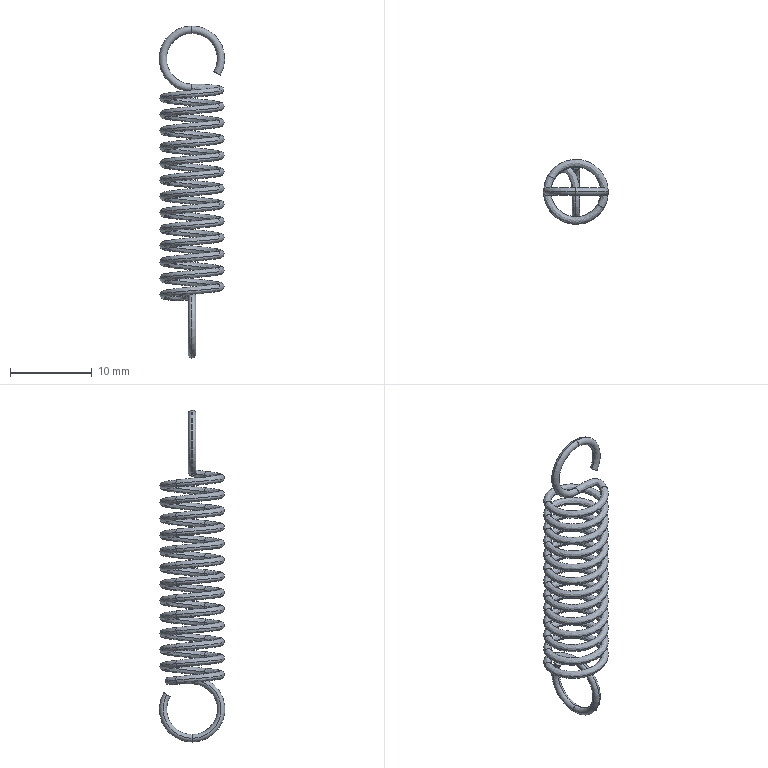Part | CATIA | 1 solid | 72 faces | box 8 x 8 x 40.5 mm | volume 205.926 mm3 | spline 54 | torus 16 | plane 2